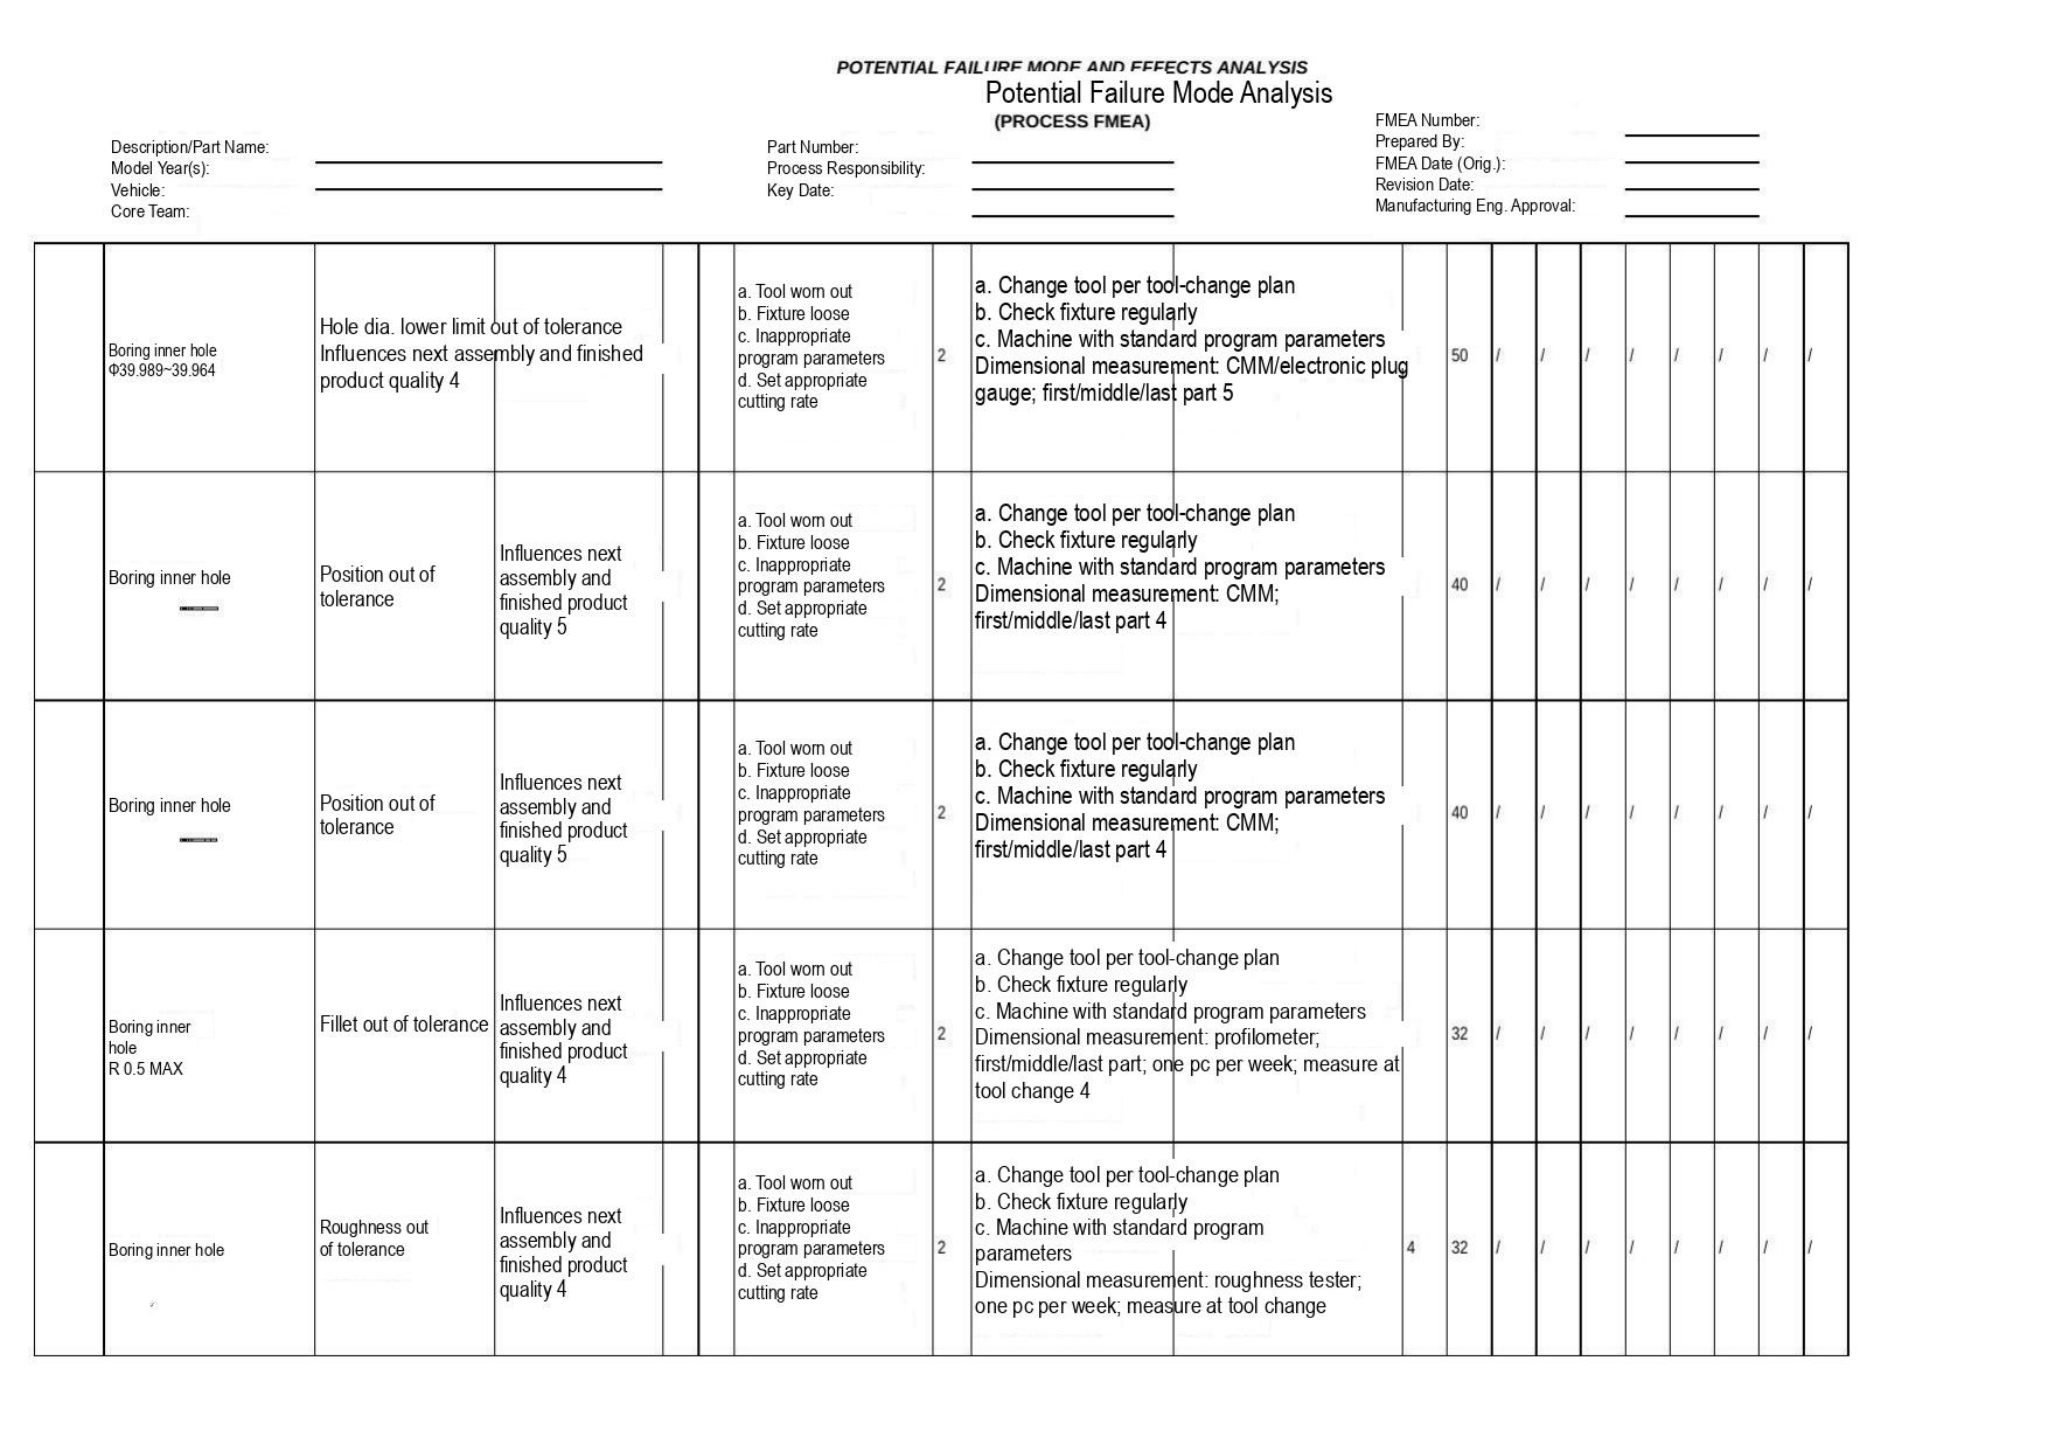POTENTIAL FAILURE MODE AND EFFECTS ANALYSIS
Potential Failure Mode Analysis
(PROCESS FMEA)

Description/Part Name:
Model Year(s):
Vehicle:
Core Team:

Part Number:
Process Responsibility:
Key Date:

FMEA Number:
Prepared By:
FMEA Date (Orig.):
Revision Date:
Manufacturing Eng. Approval:

| | | | | | | | | | | | | | | | | | | |
|---|---|---|---|---|---|---|---|---|---|---|---|---|---|---|---|---|---|---|
| | Boring inner hole Φ39.989~39.964 | Hole dia. lower limit out of tolerance | Influences next assembly and finished product quality 4 | | | a. Tool worn out<br>b. Fixture loose<br>c. Inappropriate program parameters<br>d. Set appropriate cutting rate | 2 | a. Change tool per tool-change plan<br>b. Check fixture regularly<br>c. Machine with standard program parameters<br>Dimensional measurement: CMM/electronic plug gauge; first/middle/last part 5 | | 50 | / | / | / | / | / | / | / | / |
| | Boring inner hole | Position out of tolerance | Influences next assembly and finished product quality 5 | | | a. Tool worn out<br>b. Fixture loose<br>c. Inappropriate program parameters<br>d. Set appropriate cutting rate | 2 | a. Change tool per tool-change plan<br>b. Check fixture regularly<br>c. Machine with standard program parameters<br>Dimensional measurement: CMM;<br>first/middle/last part 4 | | 40 | / | / | / | / | / | / | / | / |
| | Boring inner hole | Position out of tolerance | Influences next assembly and finished product quality 5 | | | a. Tool worn out<br>b. Fixture loose<br>c. Inappropriate program parameters<br>d. Set appropriate cutting rate | 2 | a. Change tool per tool-change plan<br>b. Check fixture regularly<br>c. Machine with standard program parameters<br>Dimensional measurement: CMM;<br>first/middle/last part 4 | | 40 | / | / | / | / | / | / | / | / |
| | Boring inner hole R 0.5 MAX | Fillet out of tolerance | Influences next assembly and finished product quality 4 | | | a. Tool worn out<br>b. Fixture loose<br>c. Inappropriate program parameters<br>d. Set appropriate cutting rate | 2 | a. Change tool per tool-change plan<br>b. Check fixture regularly<br>c. Machine with standard program parameters<br>Dimensional measurement: profilometer; first/middle/last part; one pc per week; measure at tool change 4 | | 32 | / | / | / | / | / | / | / | / |
| | Boring inner hole | Roughness out of tolerance | Influences next assembly and finished product quality 4 | | | a. Tool worn out<br>b. Fixture loose<br>c. Inappropriate program parameters<br>d. Set appropriate cutting rate | 2 | a. Change tool per tool-change plan<br>b. Check fixture regularly<br>c. Machine with standard program parameters<br>Dimensional measurement: roughness tester; one pc per week; measure at tool change | 4 | 32 | / | / | / | / | / | / | / | / |
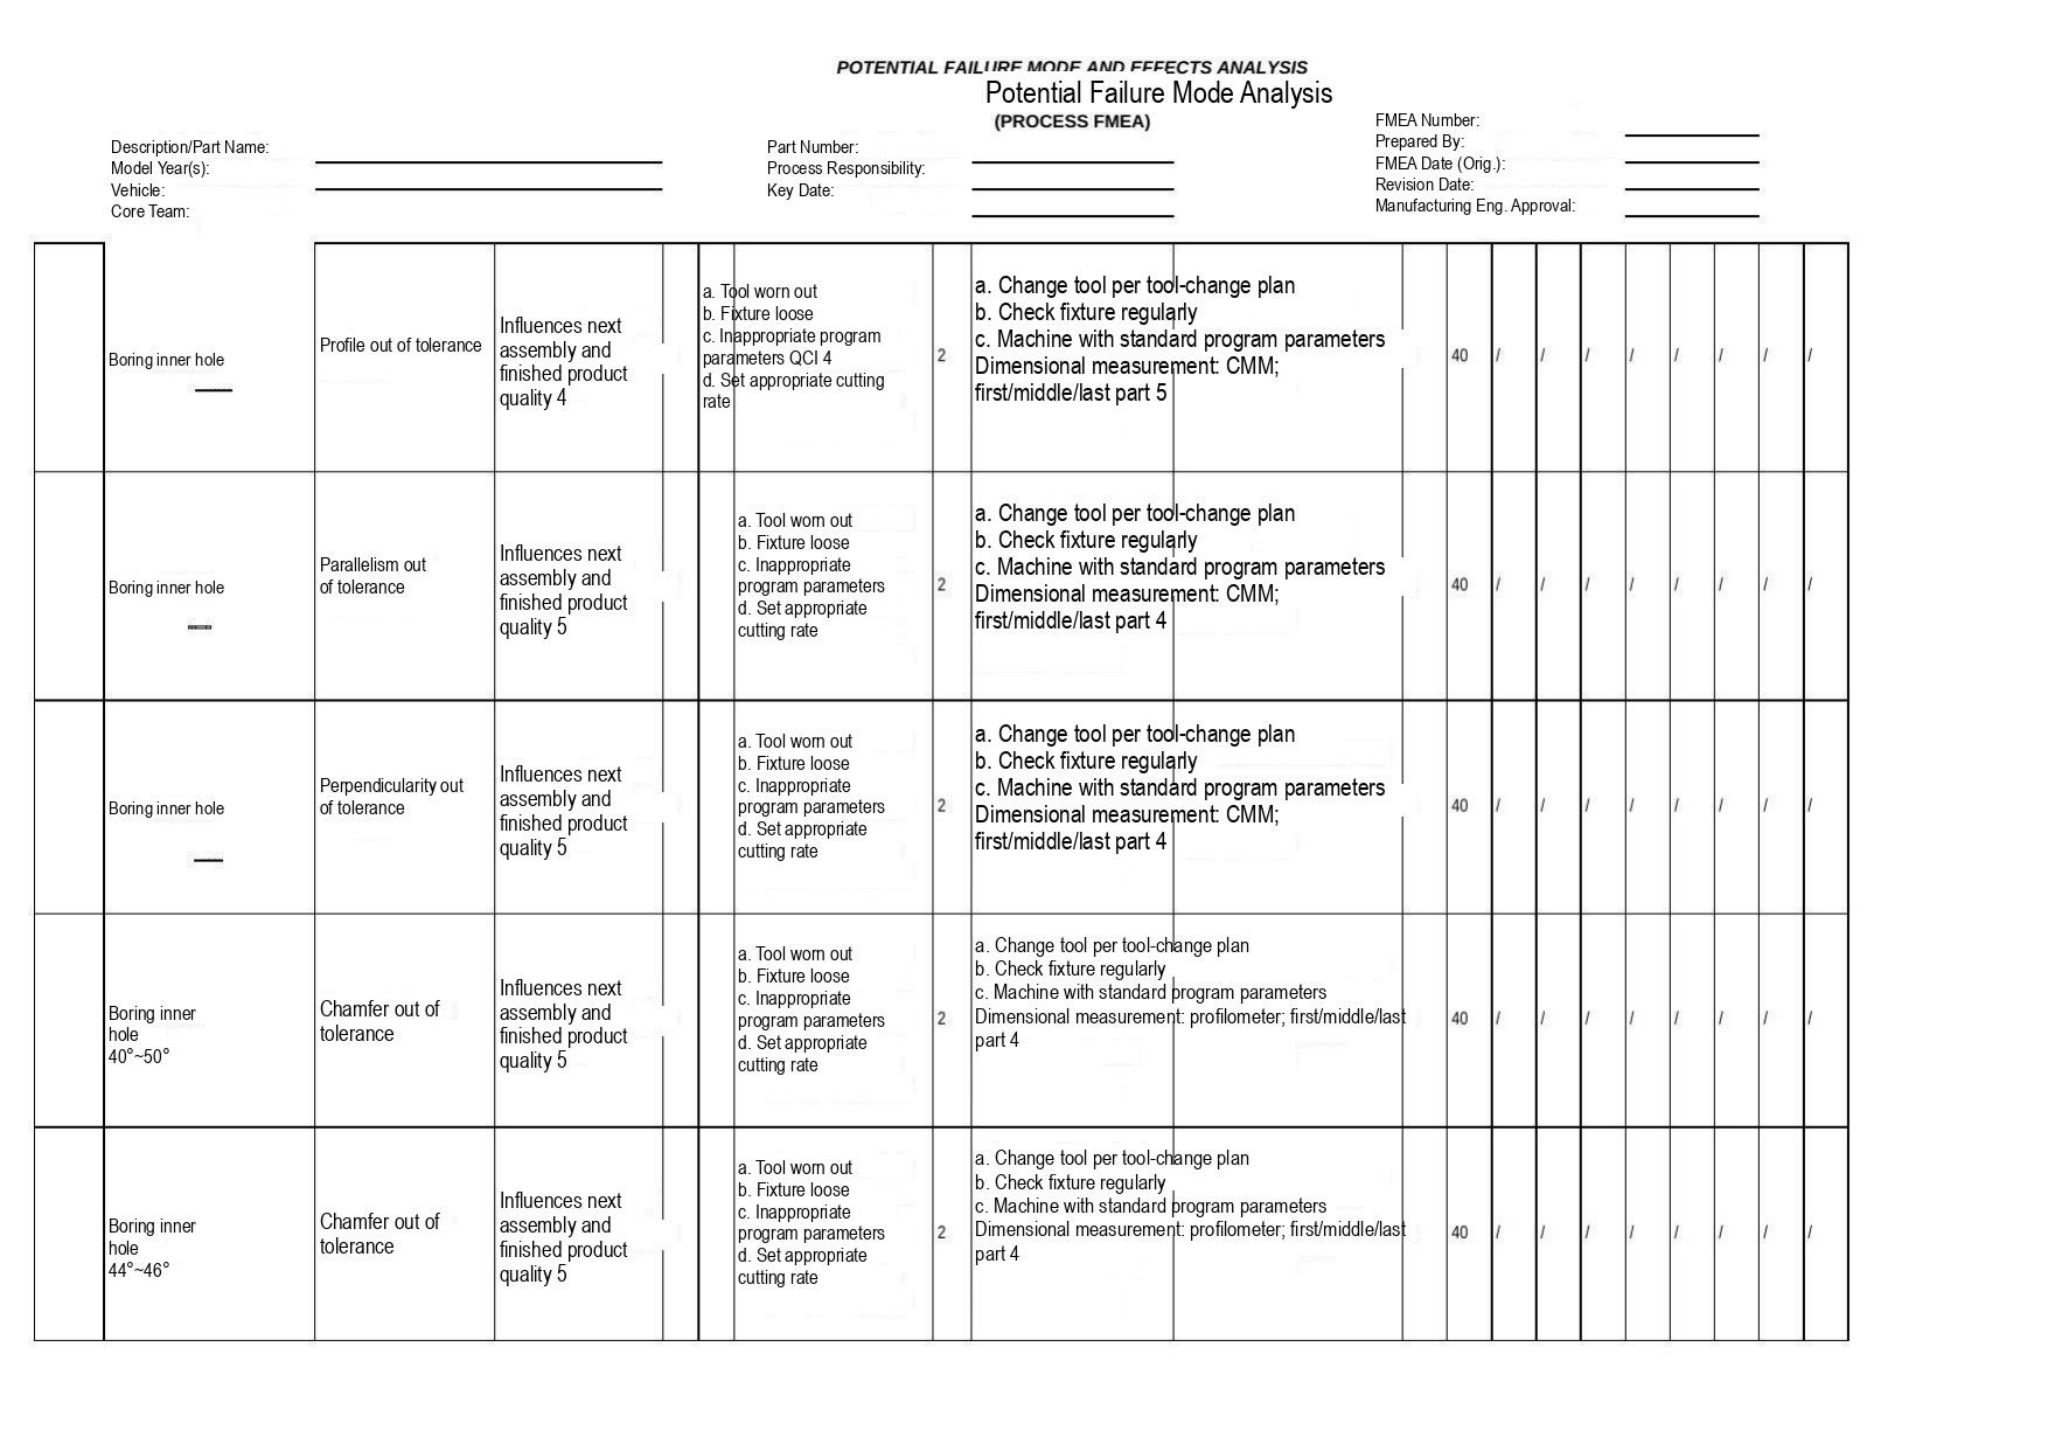POTENTIAL FAILURE MODE AND EFFECTS ANALYSIS
Potential Failure Mode Analysis
(PROCESS FMEA)

Description/Part Name:
Model Year(s):
Vehicle:
Core Team:

Part Number:
Process Responsibility:
Key Date:

FMEA Number:
Prepared By:
FMEA Date (Orig.):
Revision Date:
Manufacturing Eng. Approval:

| | | | | | | | | | | | | | | | | | | | | |
|---|---|---|---|---|---|---|---|---|---|---|---|---|---|---|---|---|---|---|---|---|
| | Boring inner hole | Profile out of tolerance | Influences next assembly and finished product quality 4 | | a. Tool worn out b. Fixture loose c. Inappropriate program parameters QCI 4 d. Set appropriate cutting rate | | 2 | a. Change tool per tool-change plan b. Check fixture regularly c. Machine with standard program parameters Dimensional measurement: CMM; first/middle/last part 5 | | | 40 | / | / | / | / | / | / | / | / | |
| | Boring inner hole | Parallelism out of tolerance | Influences next assembly and finished product quality 5 | | | a. Tool worn out b. Fixture loose c. Inappropriate program parameters d. Set appropriate cutting rate | 2 | a. Change tool per tool-change plan b. Check fixture regularly c. Machine with standard program parameters Dimensional measurement: CMM; first/middle/last part 4 | | | 40 | / | / | / | / | / | / | / | / | |
| | Boring inner hole | Perpendicularity out of tolerance | Influences next assembly and finished product quality 5 | | | a. Tool worn out b. Fixture loose c. Inappropriate program parameters d. Set appropriate cutting rate | 2 | a. Change tool per tool-change plan b. Check fixture regularly c. Machine with standard program parameters Dimensional measurement: CMM; first/middle/last part 4 | | | 40 | / | / | / | / | / | / | / | / | |
| | Boring inner hole 40°~50° | Chamfer out of tolerance | Influences next assembly and finished product quality 5 | | | a. Tool worn out b. Fixture loose c. Inappropriate program parameters d. Set appropriate cutting rate | 2 | a. Change tool per tool-change plan b. Check fixture regularly c. Machine with standard program parameters Dimensional measurement: profilometer; first/middle/last part 4 | | | 40 | / | / | / | / | / | / | / | / | |
| | Boring inner hole 44°~46° | Chamfer out of tolerance | Influences next assembly and finished product quality 5 | | | a. Tool worn out b. Fixture loose c. Inappropriate program parameters d. Set appropriate cutting rate | 2 | a. Change tool per tool-change plan b. Check fixture regularly c. Machine with standard program parameters Dimensional measurement: profilometer; first/middle/last part 4 | | | 40 | / | / | / | / | / | / | / | / | |
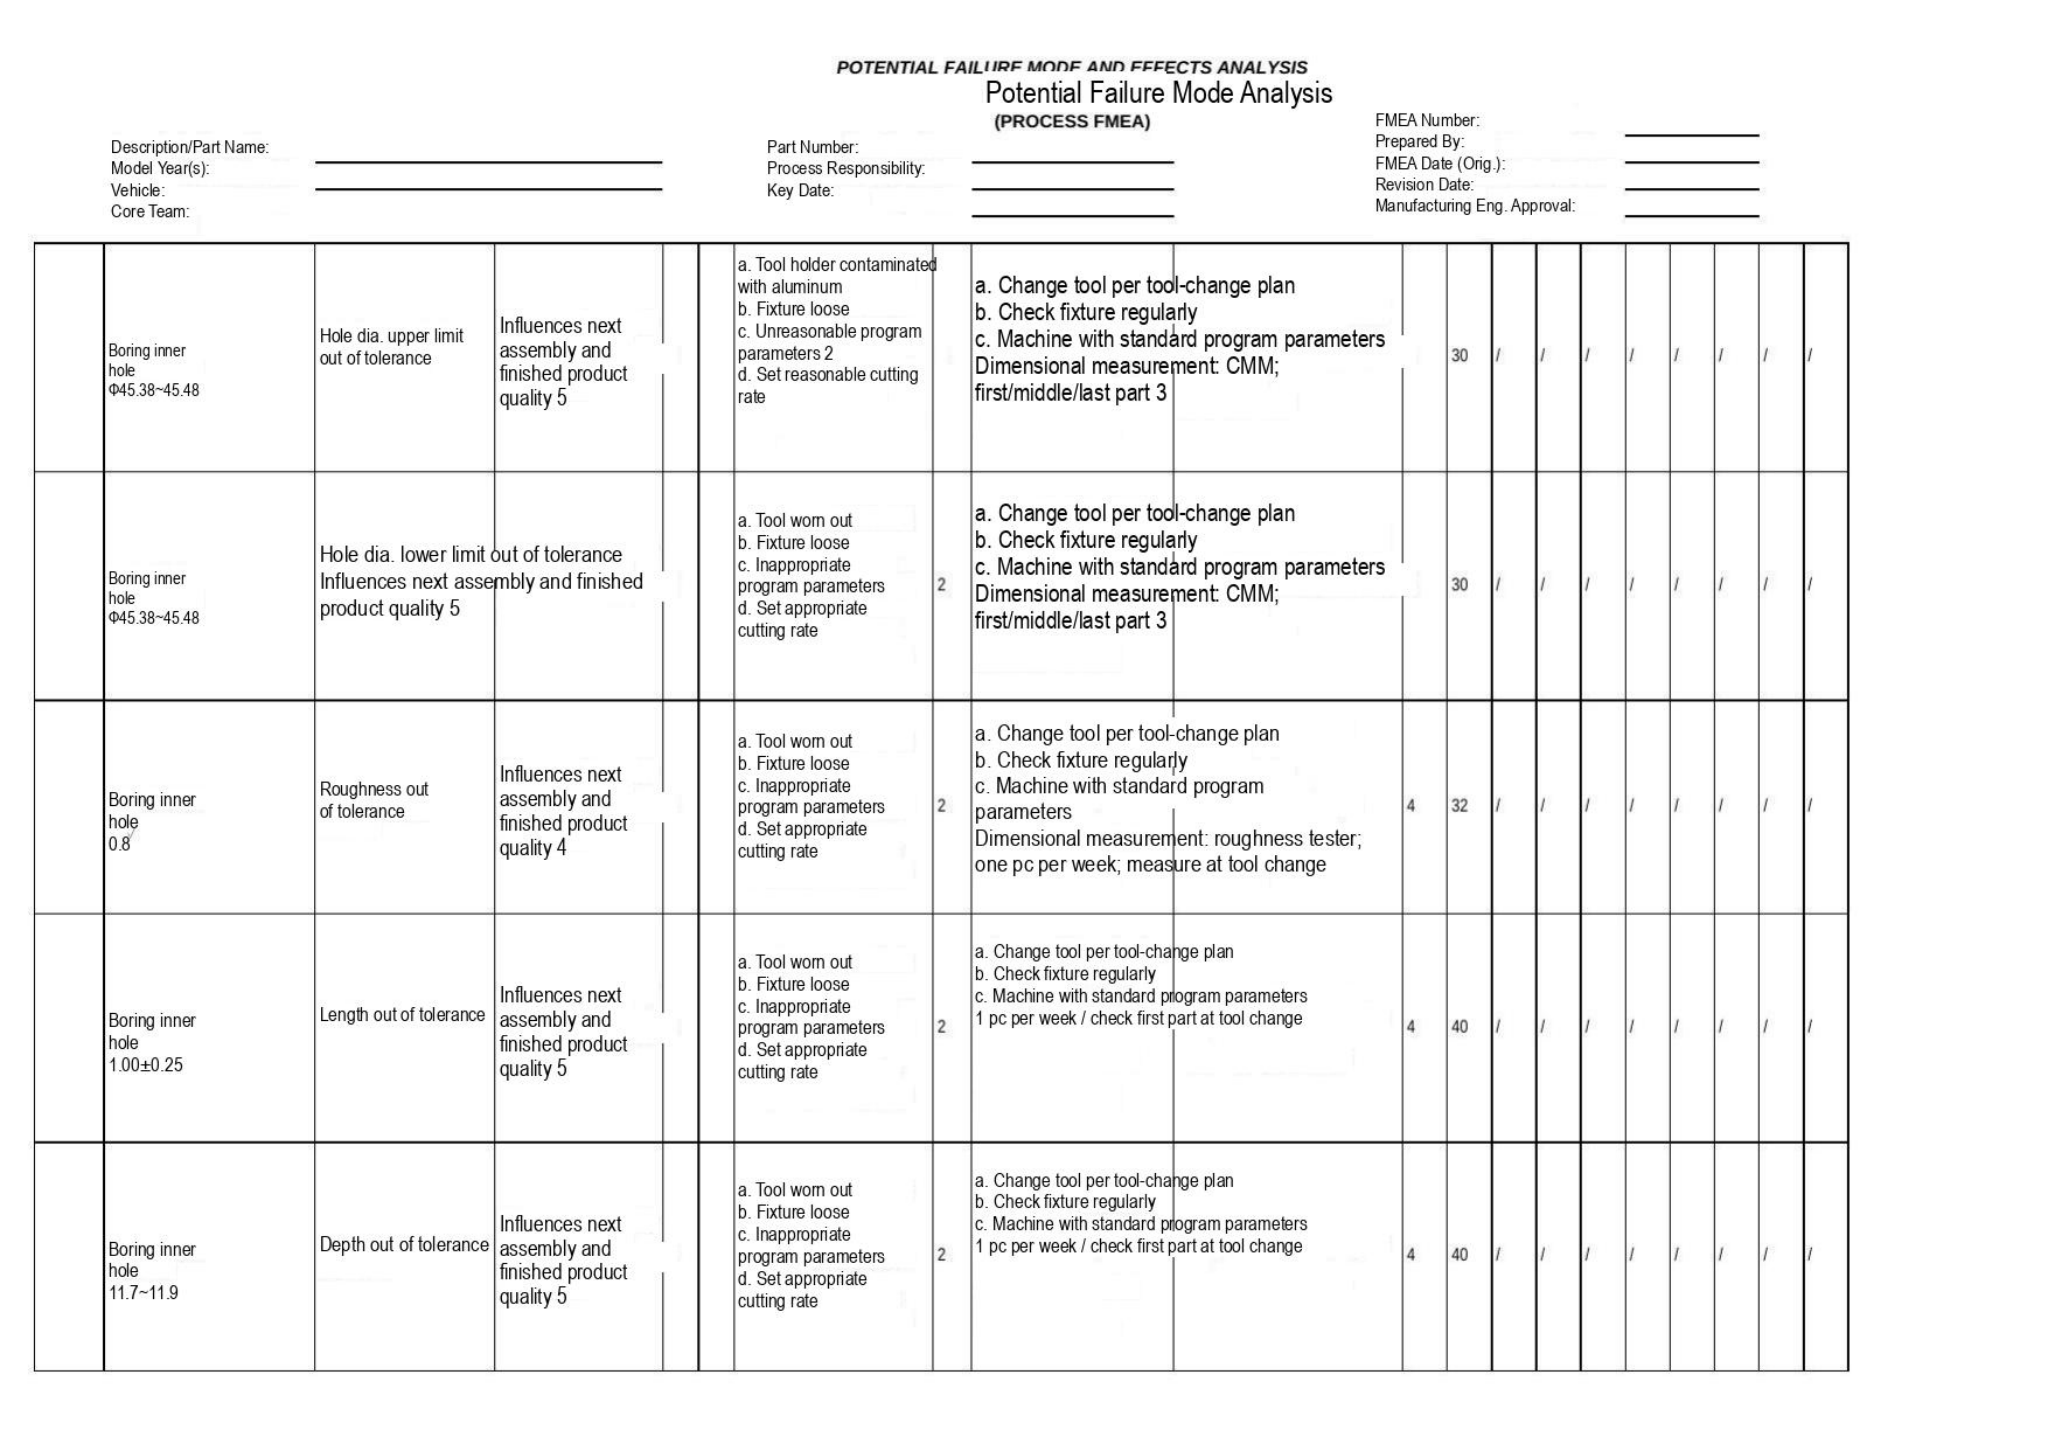POTENTIAL FAILURE MODE AND EFFECTS ANALYSIS
Potential Failure Mode Analysis
(PROCESS FMEA)

Description/Part Name:
Model Year(s):
Vehicle:
Core Team:

Part Number:
Process Responsibility:
Key Date:

FMEA Number:
Prepared By:
FMEA Date (Orig.):
Revision Date:
Manufacturing Eng. Approval:

| | | | | | | | | | | | | | | | | | | |
|---|---|---|---|---|---|---|---|---|---|---|---|---|---|---|---|---|---|---|
| | Boring inner hole Φ45.38~45.48 | Hole dia. upper limit out of tolerance | Influences next assembly and finished product quality 5 | | | a. Tool holder contaminated with aluminum<br>b. Fixture loose<br>c. Unreasonable program parameters 2<br>d. Set reasonable cutting rate | | a. Change tool per tool-change plan<br>b. Check fixture regularly<br>c. Machine with standard program parameters<br>Dimensional measurement: CMM; first/middle/last part 3 | | 30 | / | / | / | / | / | / | / | / |
| | Boring inner hole Φ45.38~45.48 | Hole dia. lower limit out of tolerance Influences next assembly and finished product quality 5 | | | | a. Tool worn out<br>b. Fixture loose<br>c. Inappropriate program parameters<br>d. Set appropriate cutting rate | 2 | a. Change tool per tool-change plan<br>b. Check fixture regularly<br>c. Machine with standard program parameters<br>Dimensional measurement: CMM; first/middle/last part 3 | | 30 | / | / | / | / | / | / | / | / |
| | Boring inner hole 0.8 | Roughness out of tolerance | Influences next assembly and finished product quality 4 | | | a. Tool worn out<br>b. Fixture loose<br>c. Inappropriate program parameters<br>d. Set appropriate cutting rate | 2 | a. Change tool per tool-change plan<br>b. Check fixture regularly<br>c. Machine with standard program parameters<br>Dimensional measurement: roughness tester; one pc per week; measure at tool change | 4 | 32 | / | / | / | / | / | / | / | / |
| | Boring inner hole 1.00±0.25 | Length out of tolerance | Influences next assembly and finished product quality 5 | | | a. Tool worn out<br>b. Fixture loose<br>c. Inappropriate program parameters<br>d. Set appropriate cutting rate | 2 | a. Change tool per tool-change plan<br>b. Check fixture regularly<br>c. Machine with standard program parameters<br>1 pc per week / check first part at tool change | 4 | 40 | / | / | / | / | / | / | / | / |
| | Boring inner hole 11.7~11.9 | Depth out of tolerance | Influences next assembly and finished product quality 5 | | | a. Tool worn out<br>b. Fixture loose<br>c. Inappropriate program parameters<br>d. Set appropriate cutting rate | 2 | a. Change tool per tool-change plan<br>b. Check fixture regularly<br>c. Machine with standard program parameters<br>1 pc per week / check first part at tool change | 4 | 40 | / | / | / | / | / | / | / | / |
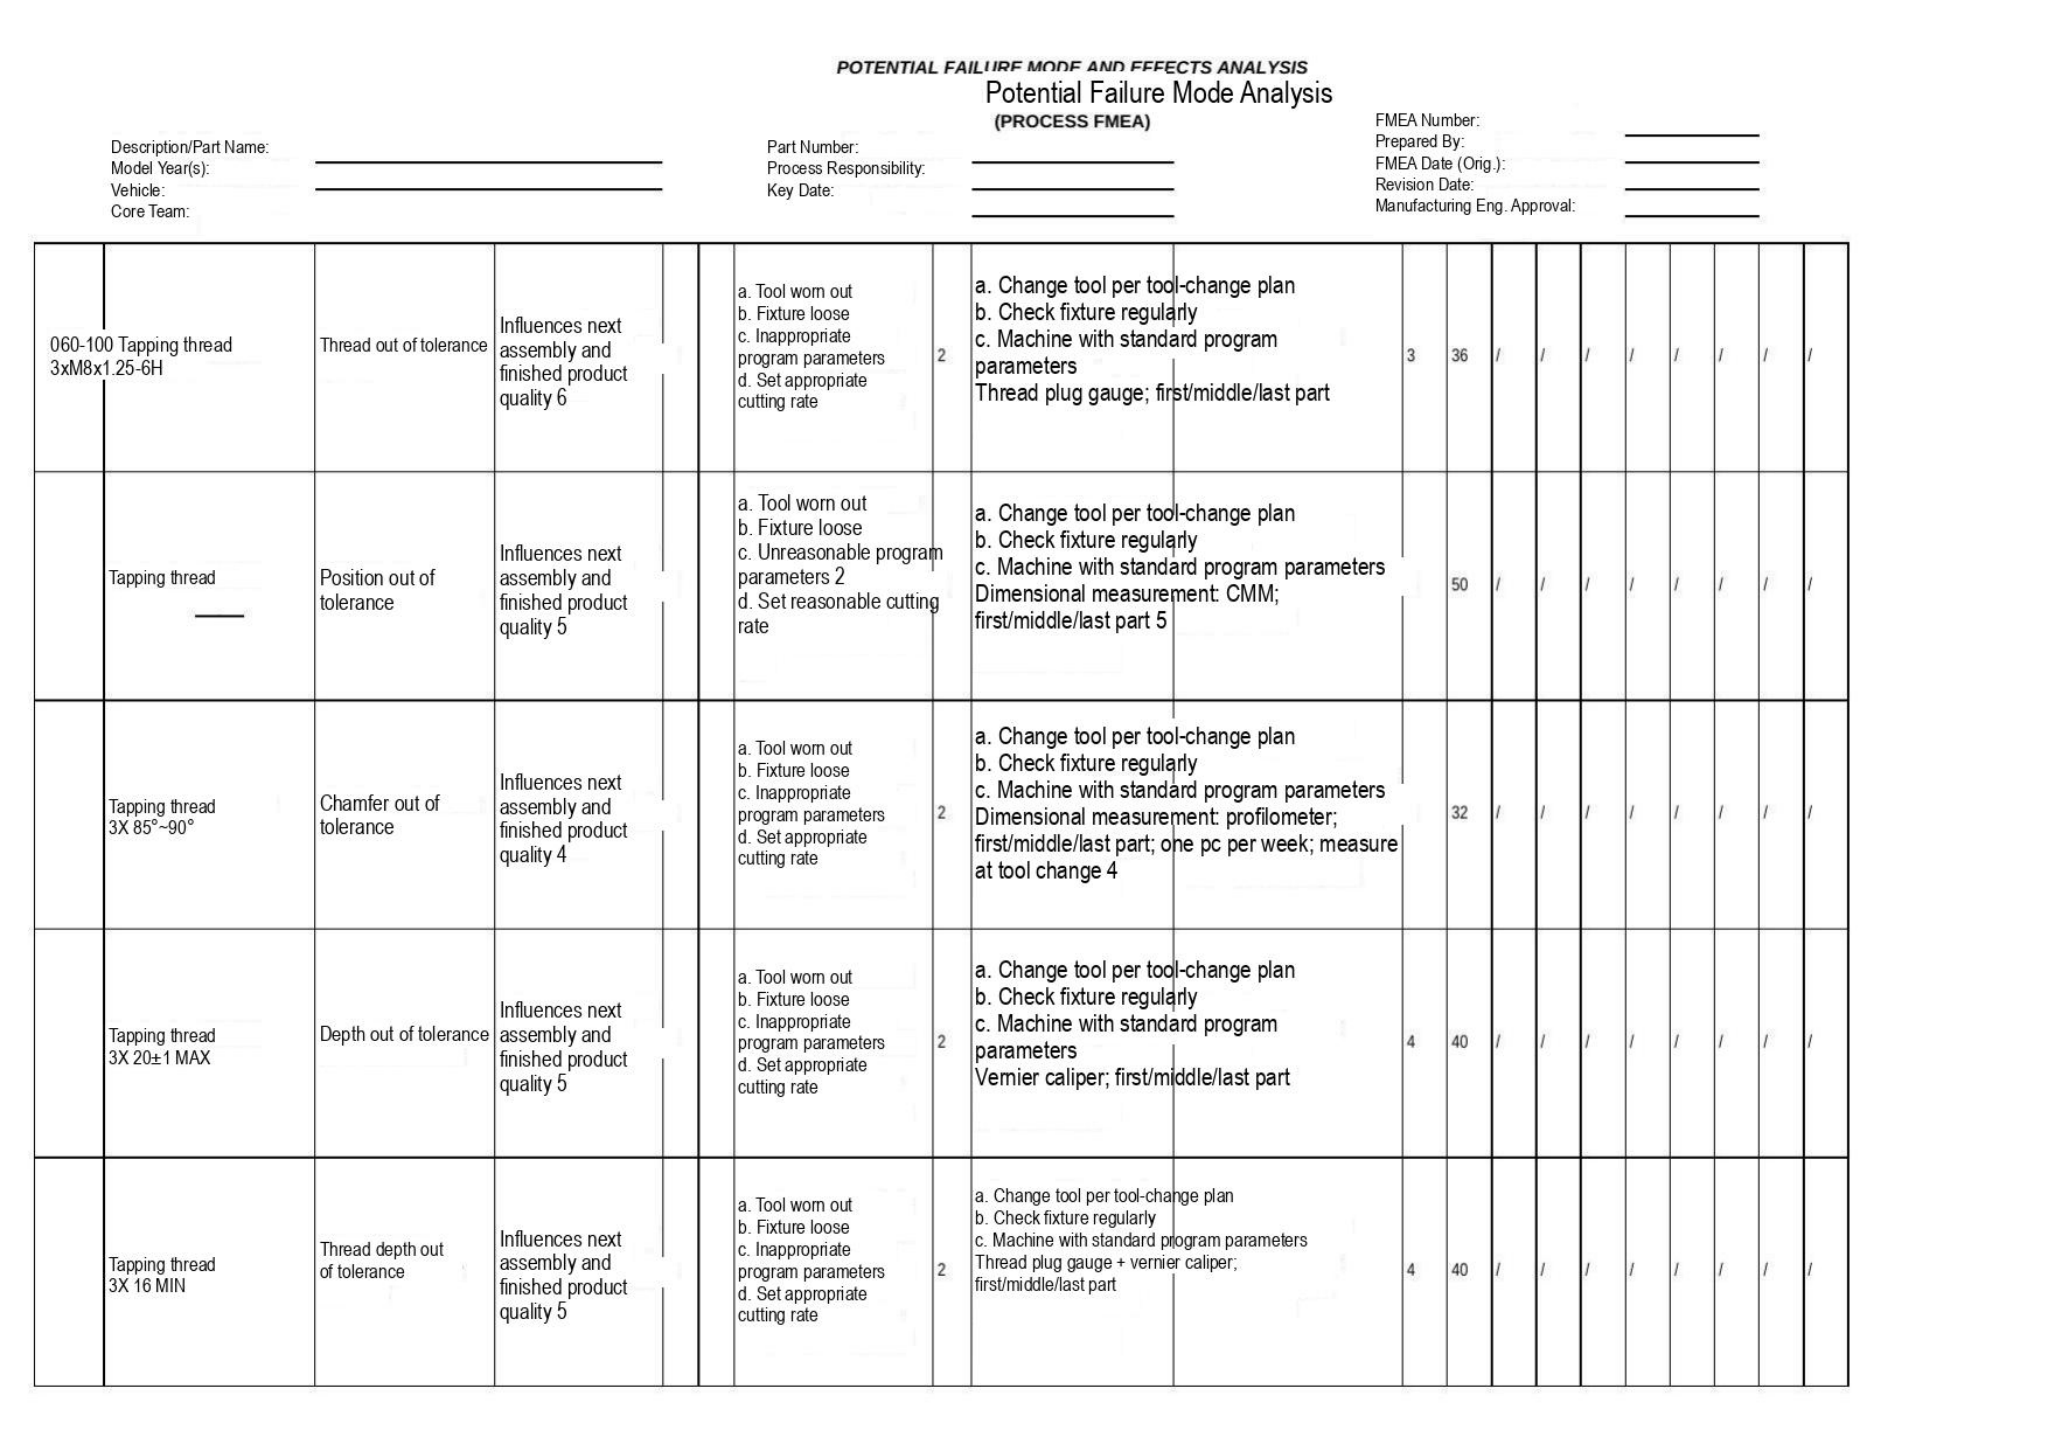POTENTIAL FAILURE MODE AND EFFECTS ANALYSIS
Potential Failure Mode Analysis
(PROCESS FMEA)

Description/Part Name:
Model Year(s):
Vehicle:
Core Team:

Part Number:
Process Responsibility:
Key Date:

FMEA Number:
Prepared By:
FMEA Date (Orig.):
Revision Date:
Manufacturing Eng. Approval:

| | | | | | | | | | | | | | | | | | | |
|---|---|---|---|---|---|---|---|---|---|---|---|---|---|---|---|---|---|---|
| 060-100 Tapping thread 3xM8x1.25-6H | | Thread out of tolerance | Influences next assembly and finished product quality 6 | | | a. Tool worn out<br>b. Fixture loose<br>c. Inappropriate program parameters<br>d. Set appropriate cutting rate | 2 | a. Change tool per tool-change plan<br>b. Check fixture regularly<br>c. Machine with standard program parameters<br>Thread plug gauge; first/middle/last part | 3 | 36 | / | / | / | / | / | / | / | / |
| | Tapping thread | Position out of tolerance | Influences next assembly and finished product quality 5 | | | a. Tool worn out<br>b. Fixture loose<br>c. Unreasonable program parameters 2<br>d. Set reasonable cutting rate | | a. Change tool per tool-change plan<br>b. Check fixture regularly<br>c. Machine with standard program parameters<br>Dimensional measurement: CMM; first/middle/last part 5 | | 50 | / | / | / | / | / | / | / | / |
| | Tapping thread 3X 85°~90° | Chamfer out of tolerance | Influences next assembly and finished product quality 4 | | | a. Tool worn out<br>b. Fixture loose<br>c. Inappropriate program parameters<br>d. Set appropriate cutting rate | 2 | a. Change tool per tool-change plan<br>b. Check fixture regularly<br>c. Machine with standard program parameters<br>Dimensional measurement: profilometer; first/middle/last part; one pc per week; measure at tool change 4 | | 32 | / | / | / | / | / | / | / | / |
| | Tapping thread 3X 20±1 MAX | Depth out of tolerance | Influences next assembly and finished product quality 5 | | | a. Tool worn out<br>b. Fixture loose<br>c. Inappropriate program parameters<br>d. Set appropriate cutting rate | 2 | a. Change tool per tool-change plan<br>b. Check fixture regularly<br>c. Machine with standard program parameters<br>Vernier caliper; first/middle/last part | 4 | 40 | / | / | / | / | / | / | / | / |
| | Tapping thread 3X 16 MIN | Thread depth out of tolerance | Influences next assembly and finished product quality 5 | | | a. Tool worn out<br>b. Fixture loose<br>c. Inappropriate program parameters<br>d. Set appropriate cutting rate | 2 | a. Change tool per tool-change plan<br>b. Check fixture regularly<br>c. Machine with standard program parameters<br>Thread plug gauge + vernier caliper; first/middle/last part | 4 | 40 | / | / | / | / | / | / | / | / |
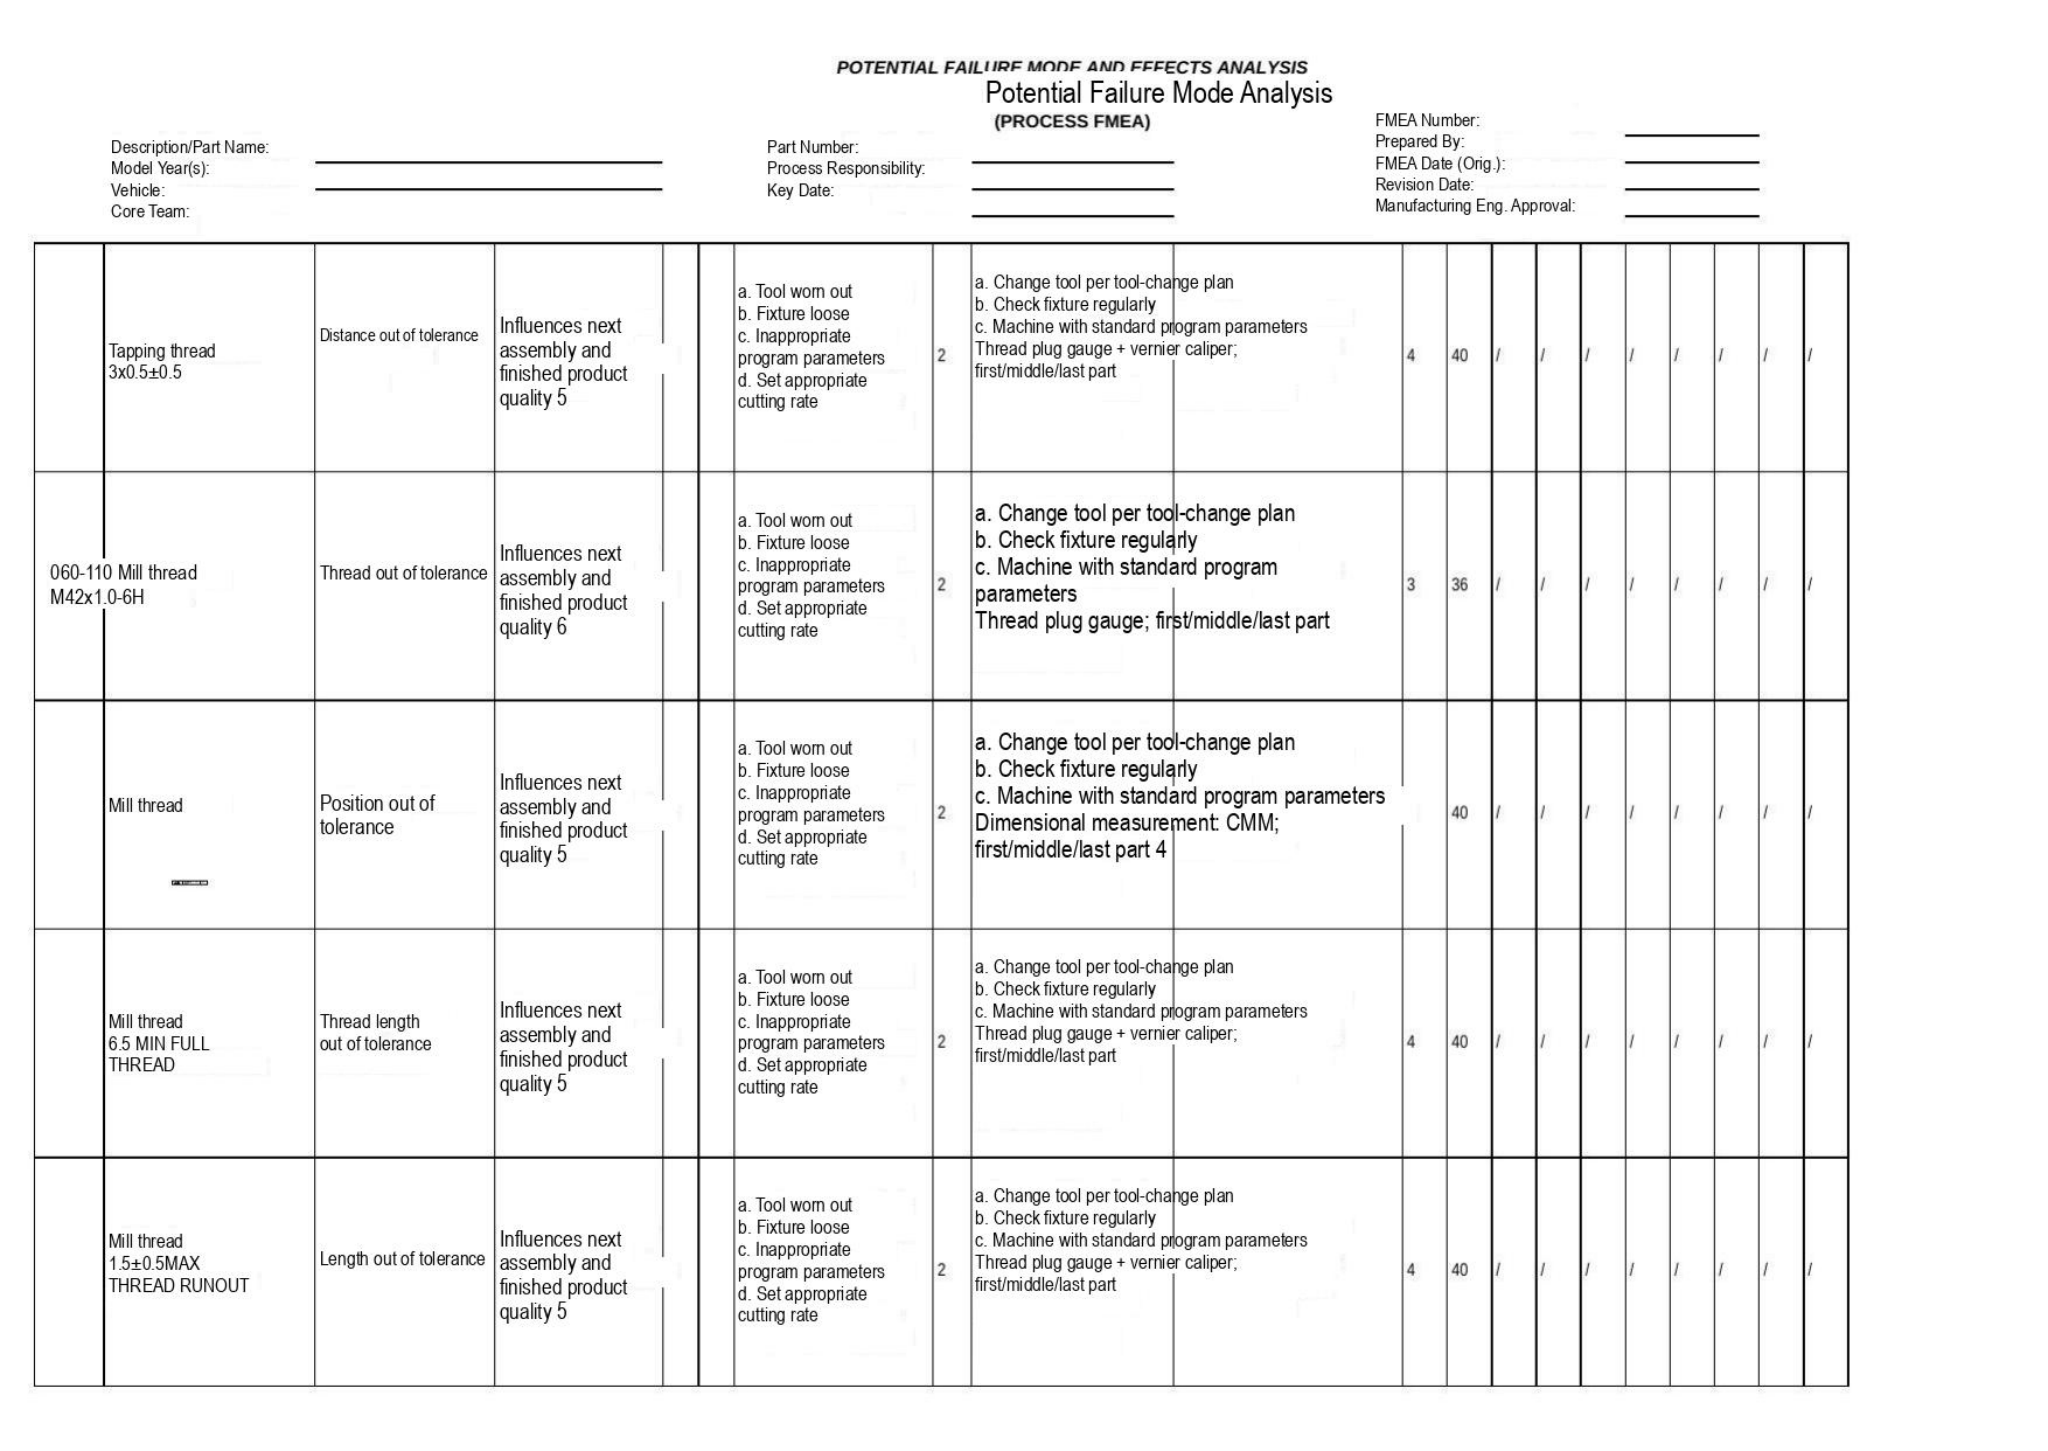**POTENTIAL FAILURE MODE AND EFFECTS ANALYSIS**

Potential Failure Mode Analysis

**(PROCESS FMEA)**

Description/Part Name: ______________________
Model Year(s): ______________________
Vehicle: ______________________
Core Team:

Part Number: ______________________
Process Responsibility: ______________________
Key Date: ______________________

FMEA Number: ______________________
Prepared By: ______________________
FMEA Date (Orig.): ______________________
Revision Date: ______________________
Manufacturing Eng. Approval: ______________________

| | | | | | | | | | | | | | | | | | | |
|---|---|---|---|---|---|---|---|---|---|---|---|---|---|---|---|---|---|---|
| | Tapping thread 3x0.5±0.5 | Distance out of tolerance | Influences next assembly and finished product quality 5 | | | a. Tool worn out<br>b. Fixture loose<br>c. Inappropriate program parameters<br>d. Set appropriate cutting rate | 2 | a. Change tool per tool-change plan<br>b. Check fixture regularly<br>c. Machine with standard program parameters<br>Thread plug gauge + vernier caliper; first/middle/last part | 4 | 40 | / | / | / | / | / | / | / | / |
| 060-110 | Mill thread M42x1.0-6H | Thread out of tolerance | Influences next assembly and finished product quality 6 | | | a. Tool worn out<br>b. Fixture loose<br>c. Inappropriate program parameters<br>d. Set appropriate cutting rate | 2 | a. Change tool per tool-change plan<br>b. Check fixture regularly<br>c. Machine with standard program parameters<br>Thread plug gauge; first/middle/last part | 3 | 36 | / | / | / | / | / | / | / | / |
| | Mill thread | Position out of tolerance | Influences next assembly and finished product quality 5 | | | a. Tool worn out<br>b. Fixture loose<br>c. Inappropriate program parameters<br>d. Set appropriate cutting rate | 2 | a. Change tool per tool-change plan<br>b. Check fixture regularly<br>c. Machine with standard program parameters<br>Dimensional measurement: CMM; first/middle/last part 4 | | 40 | / | / | / | / | / | / | / | / |
| | Mill thread 6.5 MIN FULL THREAD | Thread length out of tolerance | Influences next assembly and finished product quality 5 | | | a. Tool worn out<br>b. Fixture loose<br>c. Inappropriate program parameters<br>d. Set appropriate cutting rate | 2 | a. Change tool per tool-change plan<br>b. Check fixture regularly<br>c. Machine with standard program parameters<br>Thread plug gauge + vernier caliper; first/middle/last part | 4 | 40 | / | / | / | / | / | / | / | / |
| | Mill thread 1.5±0.5MAX THREAD RUNOUT | Length out of tolerance | Influences next assembly and finished product quality 5 | | | a. Tool worn out<br>b. Fixture loose<br>c. Inappropriate program parameters<br>d. Set appropriate cutting rate | 2 | a. Change tool per tool-change plan<br>b. Check fixture regularly<br>c. Machine with standard program parameters<br>Thread plug gauge + vernier caliper; first/middle/last part | 4 | 40 | / | / | / | / | / | / | / | / |
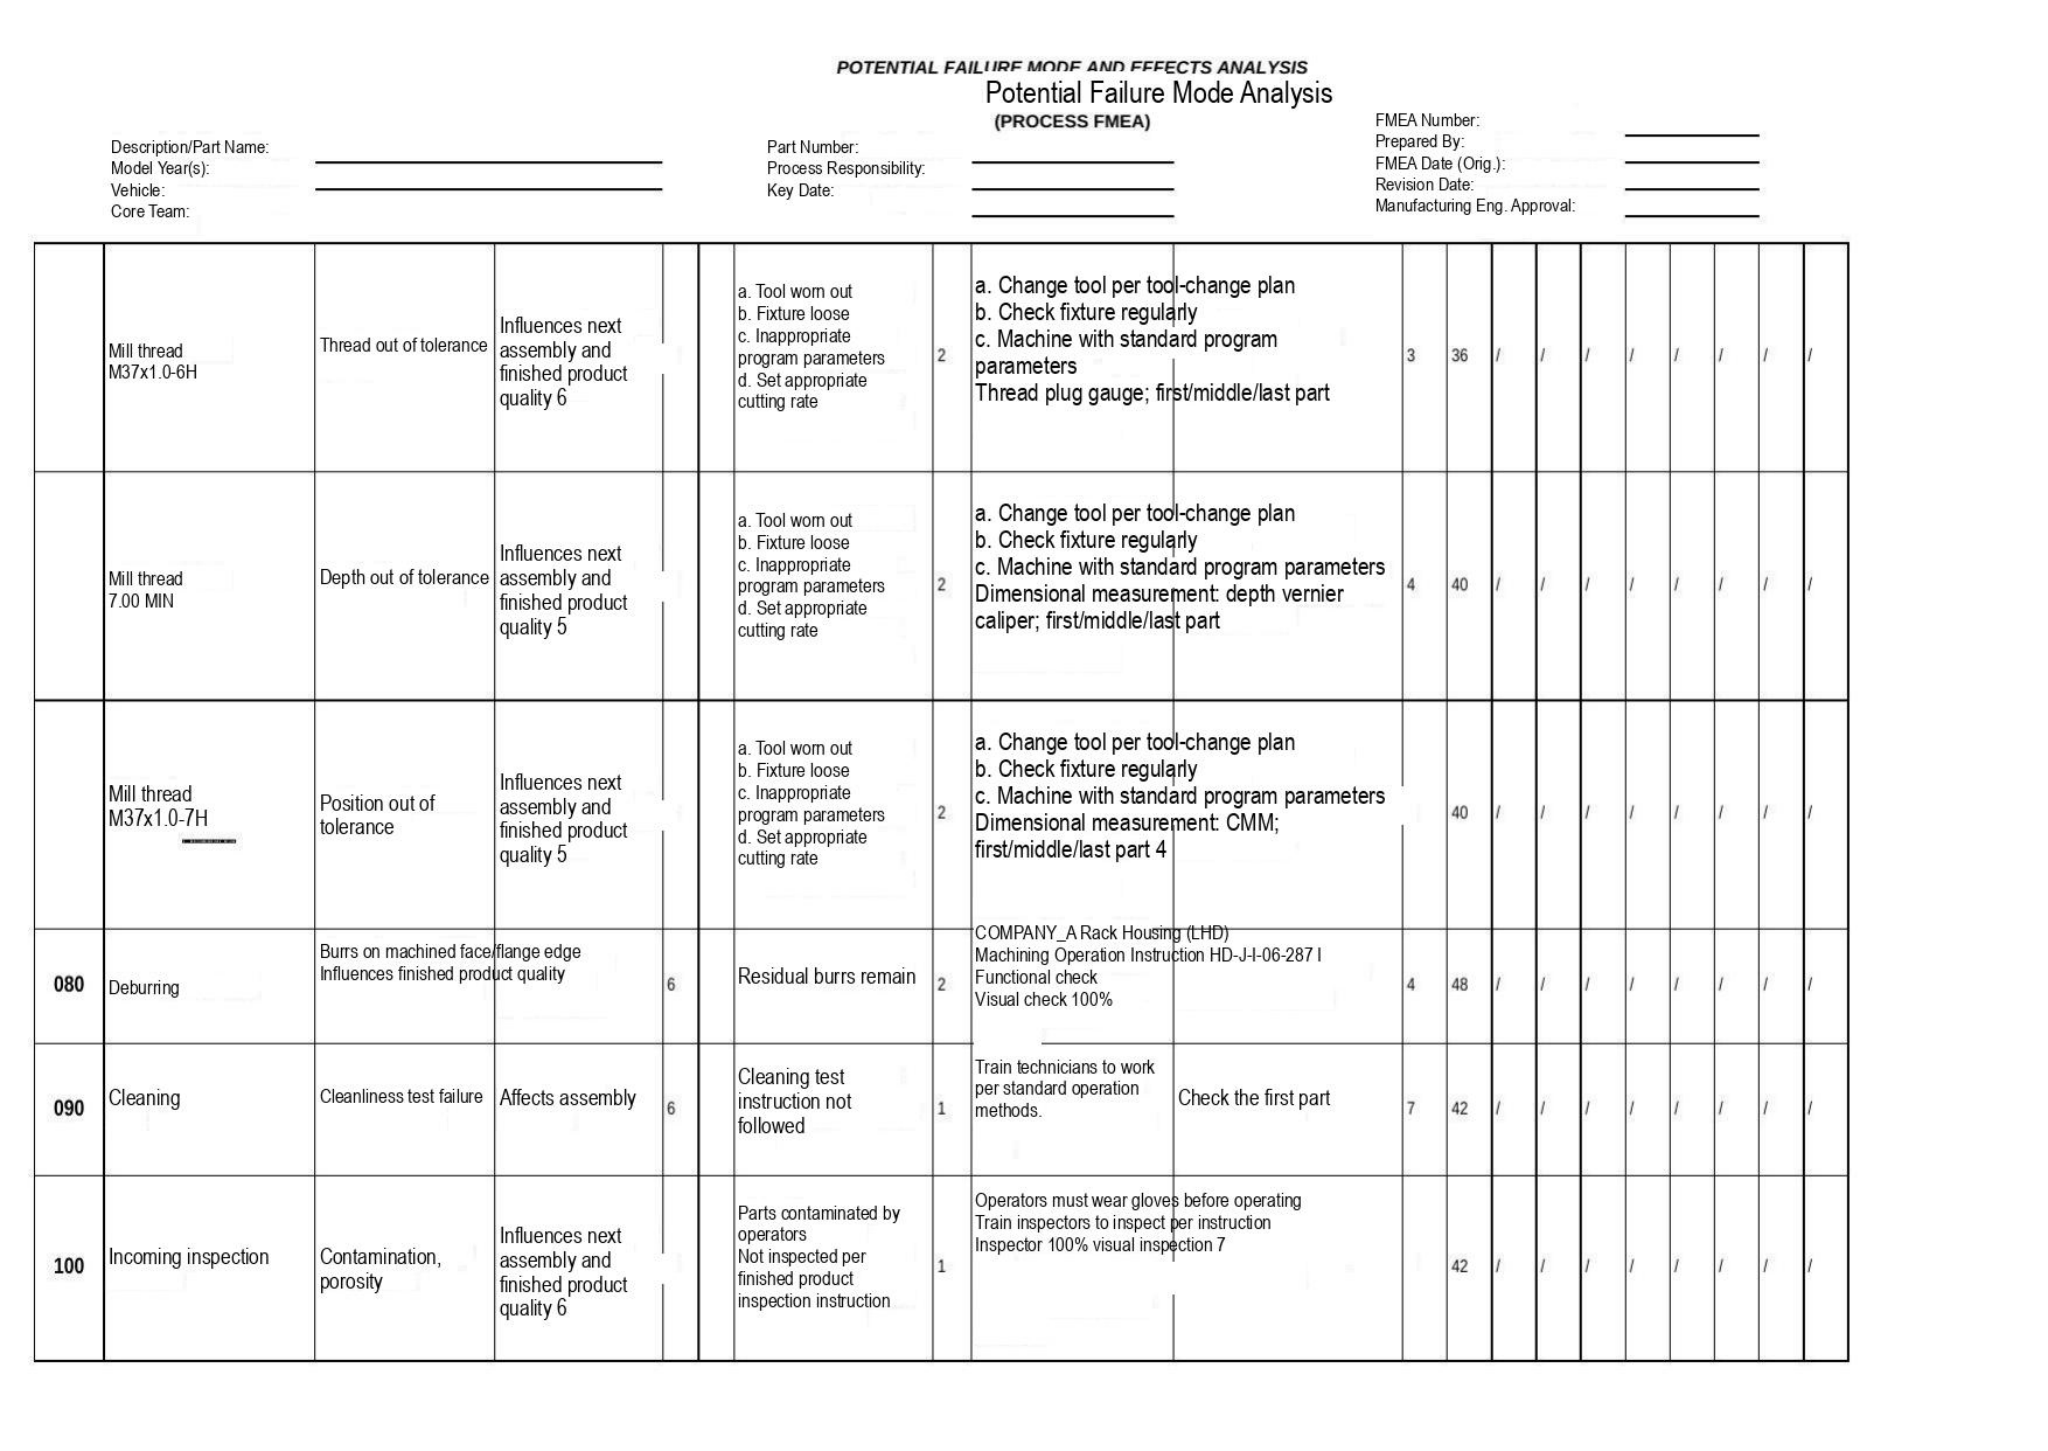POTENTIAL FAILURE MODE AND EFFECTS ANALYSIS
Potential Failure Mode Analysis
(PROCESS FMEA)

Description/Part Name:
Model Year(s):
Vehicle:
Core Team:

Part Number:
Process Responsibility:
Key Date:

FMEA Number:
Prepared By:
FMEA Date (Orig.):
Revision Date:
Manufacturing Eng. Approval:

| | | | | | | | | | | | | | | | | | | | | | |
|---|---|---|---|---|---|---|---|---|---|---|---|---|---|---|---|---|---|---|---|---|---|
| | Mill thread M37x1.0-6H | Thread out of tolerance | Influences next assembly and finished product quality 6 | | | a. Tool worn out<br>b. Fixture loose<br>c. Inappropriate program parameters<br>d. Set appropriate cutting rate | 2 | a. Change tool per tool-change plan<br>b. Check fixture regularly<br>c. Machine with standard program parameters<br>Thread plug gauge; first/middle/last part | | 3 | 36 | / | / | / | / | / | / | / | / | | |
| | Mill thread 7.00 MIN | Depth out of tolerance | Influences next assembly and finished product quality 5 | | | a. Tool worn out<br>b. Fixture loose<br>c. Inappropriate program parameters<br>d. Set appropriate cutting rate | 2 | a. Change tool per tool-change plan<br>b. Check fixture regularly<br>c. Machine with standard program parameters<br>Dimensional measurement: depth vernier caliper; first/middle/last part | | 4 | 40 | / | / | / | / | / | / | / | / | | |
| | Mill thread M37x1.0-7H | Position out of tolerance | Influences next assembly and finished product quality 5 | | | a. Tool worn out<br>b. Fixture loose<br>c. Inappropriate program parameters<br>d. Set appropriate cutting rate | 2 | a. Change tool per tool-change plan<br>b. Check fixture regularly<br>c. Machine with standard program parameters<br>Dimensional measurement: CMM; first/middle/last part 4 | | | 40 | / | / | / | / | / | / | / | / | | |
| 080 | Deburring | Burrs on machined face/flange edge<br>Influences finished product quality | | 6 | | Residual burrs remain | 2 | COMPANY_A Rack Housing (LHD)<br>Machining Operation Instruction HD-J-I-06-287 I<br>Functional check<br>Visual check 100% | | 4 | 48 | / | / | / | / | / | / | / | / | | |
| 090 | Cleaning | Cleanliness test failure | Affects assembly | 6 | | Cleaning test instruction not followed | 1 | Train technicians to work per standard operation methods. | Check the first part | 7 | 42 | / | / | / | / | / | / | / | / | | |
| 100 | Incoming inspection | Contamination, porosity | Influences next assembly and finished product quality 6 | | | Parts contaminated by operators<br>Not inspected per finished product inspection instruction | 1 | Operators must wear gloves before operating<br>Train inspectors to inspect per instruction<br>Inspector 100% visual inspection 7 | | | 42 | / | / | / | / | / | / | / | / | | |